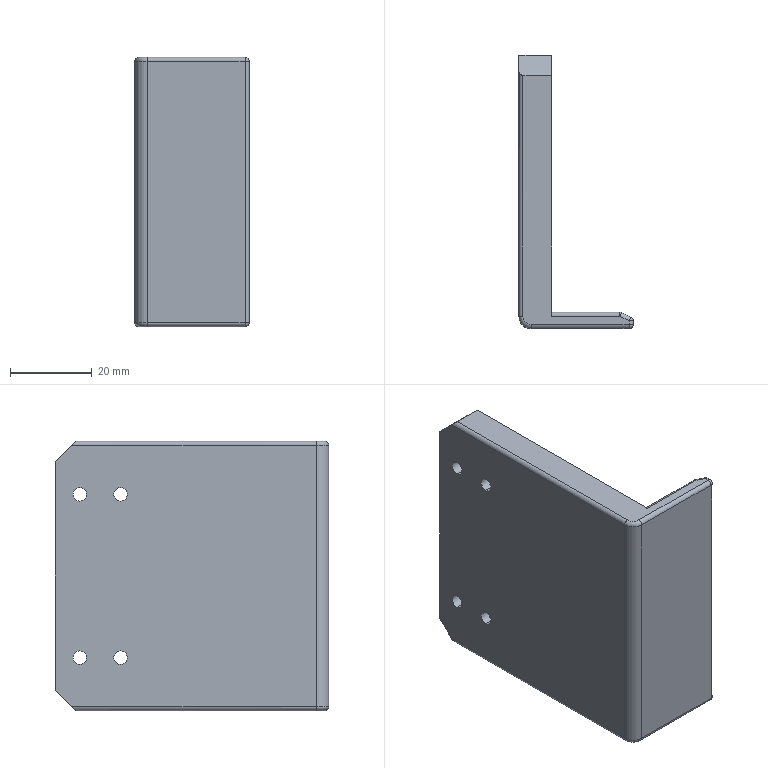Part | SolidWorks | features Fillet 3, Chamfer 2, Extrusion 1, HoleWzd 1 | 1 solid | 41 faces | box 28 x 67 x 66 mm | volume 39840 mm3 | cylinder 22 | plane 11 | sphere 6 | torus 2 | commonest cylinder face diameters 2 x13 3.3 x8 6 x1
STEP:
#1=CARTESIAN_POINT('',(8.,61.,-21.65));
#2=VERTEX_POINT('',#1);
#3=CARTESIAN_POINT('',(8.,61.,-18.35));
#4=VERTEX_POINT('',#3);
#5=CARTESIAN_POINT('',(8.,61.,-20.));
#6=DIRECTION('',(-1.,0.,0.));
#7=DIRECTION('',(0.,0.,1.));
#8=AXIS2_PLACEMENT_3D('',#5,#6,#7);
#9=CIRCLE('',#8,1.65);
#10=EDGE_CURVE('',#2,#4,#9,.T.);
#11=ORIENTED_EDGE('',*,*,#10,.F.);
#12=CARTESIAN_POINT('',(0.,61.,-21.65));
#13=VERTEX_POINT('',#12);
#14=CARTESIAN_POINT('',(0.,61.,-21.65));
#15=DIRECTION('',(-1.,0.,0.));
#16=VECTOR('',#15,1000.);
#17=LINE('',#14,#16);
#18=EDGE_CURVE('',#2,#13,#17,.T.);
#19=ORIENTED_EDGE('',*,*,#18,.T.);
#20=CARTESIAN_POINT('',(0.,61.,-18.35));
#21=VERTEX_POINT('',#20);
#22=CARTESIAN_POINT('',(0.,61.,-20.));
#23=DIRECTION('',(-1.,0.,0.));
#24=DIRECTION('',(0.,0.,1.));
#25=AXIS2_PLACEMENT_3D('',#22,#23,#24);
#26=CIRCLE('',#25,1.65);
#27=EDGE_CURVE('',#13,#21,#26,.T.);
#28=ORIENTED_EDGE('',*,*,#27,.T.);
#29=CARTESIAN_POINT('',(0.,61.,-18.35));
#30=DIRECTION('',(-1.,0.,0.));
#31=VECTOR('',#30,1000.);
#32=LINE('',#29,#31);
#33=EDGE_CURVE('',#4,#21,#32,.T.);
#34=ORIENTED_EDGE('',*,*,#33,.F.);
#35=EDGE_LOOP('',(#11,#19,#28,#34));
#36=FACE_OUTER_BOUND('',#35,.T.);
#37=CARTESIAN_POINT('',(0.,61.,-20.));
#38=DIRECTION('',(-1.,0.,0.));
#39=DIRECTION('',(0.,0.,1.));
#40=AXIS2_PLACEMENT_3D('',#37,#38,#39);
#41=CYLINDRICAL_SURFACE('',#40,1.65);
#42=ADVANCED_FACE('',(#36),#41,.F.);
#43=CARTESIAN_POINT('',(8.,61.,18.35));
#44=VERTEX_POINT('',#43);
#45=CARTESIAN_POINT('',(8.,61.,21.65));
#46=VERTEX_POINT('',#45);
#47=CARTESIAN_POINT('',(8.,61.,20.));
#48=DIRECTION('',(-1.,0.,0.));
#49=DIRECTION('',(0.,0.,1.));
#50=AXIS2_PLACEMENT_3D('',#47,#48,#49);
#51=CIRCLE('',#50,1.65);
#52=EDGE_CURVE('',#44,#46,#51,.T.);
#53=ORIENTED_EDGE('',*,*,#52,.F.);
#54=CARTESIAN_POINT('',(0.,61.,18.35));
#55=VERTEX_POINT('',#54);
#56=CARTESIAN_POINT('',(0.,61.,18.35));
#57=DIRECTION('',(-1.,0.,0.));
#58=VECTOR('',#57,1000.);
#59=LINE('',#56,#58);
#60=EDGE_CURVE('',#44,#55,#59,.T.);
#61=ORIENTED_EDGE('',*,*,#60,.T.);
#62=CARTESIAN_POINT('',(0.,61.,21.65));
#63=VERTEX_POINT('',#62);
#64=CARTESIAN_POINT('',(0.,61.,20.));
#65=DIRECTION('',(-1.,0.,0.));
#66=DIRECTION('',(0.,0.,1.));
#67=AXIS2_PLACEMENT_3D('',#64,#65,#66);
#68=CIRCLE('',#67,1.65);
#69=EDGE_CURVE('',#55,#63,#68,.T.);
#70=ORIENTED_EDGE('',*,*,#69,.T.);
#71=CARTESIAN_POINT('',(0.,61.,21.65));
#72=DIRECTION('',(-1.,0.,0.));
#73=VECTOR('',#72,1000.);
#74=LINE('',#71,#73);
#75=EDGE_CURVE('',#46,#63,#74,.T.);
#76=ORIENTED_EDGE('',*,*,#75,.F.);
#77=EDGE_LOOP('',(#53,#61,#70,#76));
#78=FACE_OUTER_BOUND('',#77,.T.);
#79=CARTESIAN_POINT('',(0.,61.,20.));
#80=DIRECTION('',(-1.,0.,0.));
#81=DIRECTION('',(0.,0.,1.));
#82=AXIS2_PLACEMENT_3D('',#79,#80,#81);
#83=CYLINDRICAL_SURFACE('',#82,1.65);
#84=ADVANCED_FACE('',(#78),#83,.F.);
#85=CARTESIAN_POINT('',(8.,51.,-21.65));
#86=VERTEX_POINT('',#85);
#87=CARTESIAN_POINT('',(8.,51.,-18.35));
#88=VERTEX_POINT('',#87);
#89=CARTESIAN_POINT('',(8.,51.,-20.));
#90=DIRECTION('',(-1.,0.,0.));
#91=DIRECTION('',(0.,0.,1.));
#92=AXIS2_PLACEMENT_3D('',#89,#90,#91);
#93=CIRCLE('',#92,1.65);
#94=EDGE_CURVE('',#86,#88,#93,.T.);
#95=ORIENTED_EDGE('',*,*,#94,.F.);
#96=CARTESIAN_POINT('',(0.,51.,-21.65));
#97=VERTEX_POINT('',#96);
#98=CARTESIAN_POINT('',(0.,51.,-21.65));
#99=DIRECTION('',(-1.,0.,0.));
#100=VECTOR('',#99,1000.);
#101=LINE('',#98,#100);
#102=EDGE_CURVE('',#86,#97,#101,.T.);
#103=ORIENTED_EDGE('',*,*,#102,.T.);
#104=CARTESIAN_POINT('',(0.,51.,-18.35));
#105=VERTEX_POINT('',#104);
#106=CARTESIAN_POINT('',(0.,51.,-20.));
#107=DIRECTION('',(-1.,0.,0.));
#108=DIRECTION('',(0.,0.,1.));
#109=AXIS2_PLACEMENT_3D('',#106,#107,#108);
#110=CIRCLE('',#109,1.65);
#111=EDGE_CURVE('',#97,#105,#110,.T.);
#112=ORIENTED_EDGE('',*,*,#111,.T.);
#113=CARTESIAN_POINT('',(0.,51.,-18.35));
#114=DIRECTION('',(-1.,0.,0.));
#115=VECTOR('',#114,1000.);
#116=LINE('',#113,#115);
#117=EDGE_CURVE('',#88,#105,#116,.T.);
#118=ORIENTED_EDGE('',*,*,#117,.F.);
#119=EDGE_LOOP('',(#95,#103,#112,#118));
#120=FACE_OUTER_BOUND('',#119,.T.);
#121=CARTESIAN_POINT('',(0.,51.,-20.));
#122=DIRECTION('',(-1.,0.,0.));
#123=DIRECTION('',(0.,0.,1.));
#124=AXIS2_PLACEMENT_3D('',#121,#122,#123);
#125=CYLINDRICAL_SURFACE('',#124,1.65);
#126=ADVANCED_FACE('',(#120),#125,.F.);
#127=CARTESIAN_POINT('',(8.,51.,18.35));
#128=VERTEX_POINT('',#127);
#129=CARTESIAN_POINT('',(8.,51.,21.65));
#130=VERTEX_POINT('',#129);
#131=CARTESIAN_POINT('',(8.,51.,20.));
#132=DIRECTION('',(-1.,0.,0.));
#133=DIRECTION('',(0.,0.,1.));
#134=AXIS2_PLACEMENT_3D('',#131,#132,#133);
#135=CIRCLE('',#134,1.65);
#136=EDGE_CURVE('',#128,#130,#135,.T.);
#137=ORIENTED_EDGE('',*,*,#136,.F.);
#138=CARTESIAN_POINT('',(0.,51.,18.35));
#139=VERTEX_POINT('',#138);
#140=CARTESIAN_POINT('',(0.,51.,18.35));
#141=DIRECTION('',(-1.,0.,0.));
#142=VECTOR('',#141,1000.);
#143=LINE('',#140,#142);
#144=EDGE_CURVE('',#128,#139,#143,.T.);
#145=ORIENTED_EDGE('',*,*,#144,.T.);
#146=CARTESIAN_POINT('',(0.,51.,21.65));
#147=VERTEX_POINT('',#146);
#148=CARTESIAN_POINT('',(0.,51.,20.));
#149=DIRECTION('',(-1.,0.,0.));
#150=DIRECTION('',(0.,0.,1.));
#151=AXIS2_PLACEMENT_3D('',#148,#149,#150);
#152=CIRCLE('',#151,1.65);
#153=EDGE_CURVE('',#139,#147,#152,.T.);
#154=ORIENTED_EDGE('',*,*,#153,.T.);
#155=CARTESIAN_POINT('',(0.,51.,21.65));
#156=DIRECTION('',(-1.,0.,0.));
#157=VECTOR('',#156,1000.);
#158=LINE('',#155,#157);
#159=EDGE_CURVE('',#130,#147,#158,.T.);
#160=ORIENTED_EDGE('',*,*,#159,.F.);
#161=EDGE_LOOP('',(#137,#145,#154,#160));
#162=FACE_OUTER_BOUND('',#161,.T.);
#163=CARTESIAN_POINT('',(0.,51.,20.));
#164=DIRECTION('',(-1.,0.,0.));
#165=DIRECTION('',(0.,0.,1.));
#166=AXIS2_PLACEMENT_3D('',#163,#164,#165);
#167=CYLINDRICAL_SURFACE('',#166,1.65);
#168=ADVANCED_FACE('',(#162),#167,.F.);
#169=CARTESIAN_POINT('',(27.,0.,-32.));
#170=VERTEX_POINT('',#169);
#171=CARTESIAN_POINT('',(27.,0.,32.));
#172=VERTEX_POINT('',#171);
#173=CARTESIAN_POINT('',(27.,0.,33.));
#174=DIRECTION('',(0.,0.,1.));
#175=VECTOR('',#174,1000.);
#176=LINE('',#173,#175);
#177=EDGE_CURVE('',#170,#172,#176,.T.);
#178=ORIENTED_EDGE('',*,*,#177,.T.);
#179=CARTESIAN_POINT('',(3.,0.,32.));
#180=VERTEX_POINT('',#179);
#181=CARTESIAN_POINT('',(3.,0.,32.));
#182=DIRECTION('',(-1.,0.,0.));
#183=VECTOR('',#182,1000.);
#184=LINE('',#181,#183);
#185=EDGE_CURVE('',#172,#180,#184,.T.);
#186=ORIENTED_EDGE('',*,*,#185,.T.);
#187=CARTESIAN_POINT('',(3.,0.,-32.));
#188=VERTEX_POINT('',#187);
#189=CARTESIAN_POINT('',(3.,0.,33.));
#190=DIRECTION('',(0.,0.,-1.));
#191=VECTOR('',#190,1000.);
#192=LINE('',#189,#191);
#193=EDGE_CURVE('',#180,#188,#192,.T.);
#194=ORIENTED_EDGE('',*,*,#193,.T.);
#195=CARTESIAN_POINT('',(0.,0.,-32.));
#196=DIRECTION('',(1.,0.,0.));
#197=VECTOR('',#196,1000.);
#198=LINE('',#195,#197);
#199=EDGE_CURVE('',#188,#170,#198,.T.);
#200=ORIENTED_EDGE('',*,*,#199,.T.);
#201=EDGE_LOOP('',(#178,#186,#194,#200));
#202=FACE_OUTER_BOUND('',#201,.T.);
#203=CARTESIAN_POINT('',(0.,0.,33.));
#204=DIRECTION('',(0.,1.,0.));
#205=DIRECTION('',(0.,0.,1.));
#206=AXIS2_PLACEMENT_3D('',#203,#204,#205);
#207=PLANE('',#206);
#208=ADVANCED_FACE('',(#202),#207,.F.);
#209=CARTESIAN_POINT('',(28.,1.882,-32.));
#210=VERTEX_POINT('',#209);
#211=CARTESIAN_POINT('',(28.,1.882,32.));
#212=VERTEX_POINT('',#211);
#213=CARTESIAN_POINT('',(28.,1.882,33.));
#214=DIRECTION('',(0.,0.,1.));
#215=VECTOR('',#214,1000.);
#216=LINE('',#213,#215);
#217=EDGE_CURVE('',#210,#212,#216,.T.);
#218=ORIENTED_EDGE('',*,*,#217,.T.);
#219=CARTESIAN_POINT('',(28.,1.,32.));
#220=VERTEX_POINT('',#219);
#221=CARTESIAN_POINT('',(28.,1.,32.));
#222=DIRECTION('',(0.,-1.,0.));
#223=VECTOR('',#222,1000.);
#224=LINE('',#221,#223);
#225=EDGE_CURVE('',#212,#220,#224,.T.);
#226=ORIENTED_EDGE('',*,*,#225,.T.);
#227=CARTESIAN_POINT('',(28.,1.,-32.));
#228=VERTEX_POINT('',#227);
#229=CARTESIAN_POINT('',(28.,1.,33.));
#230=DIRECTION('',(0.,0.,-1.));
#231=VECTOR('',#230,1000.);
#232=LINE('',#229,#231);
#233=EDGE_CURVE('',#220,#228,#232,.T.);
#234=ORIENTED_EDGE('',*,*,#233,.T.);
#235=CARTESIAN_POINT('',(28.,0.,-32.));
#236=DIRECTION('',(0.,1.,0.));
#237=VECTOR('',#236,1000.);
#238=LINE('',#235,#237);
#239=EDGE_CURVE('',#228,#210,#238,.T.);
#240=ORIENTED_EDGE('',*,*,#239,.T.);
#241=EDGE_LOOP('',(#218,#226,#234,#240));
#242=FACE_OUTER_BOUND('',#241,.T.);
#243=CARTESIAN_POINT('',(28.,0.,33.));
#244=DIRECTION('',(-1.,0.,0.));
#245=DIRECTION('',(0.,0.,1.));
#246=AXIS2_PLACEMENT_3D('',#243,#244,#245);
#247=PLANE('',#246);
#248=ADVANCED_FACE('',(#242),#247,.F.);
#249=CARTESIAN_POINT('',(8.,4.,32.));
#250=VERTEX_POINT('',#249);
#251=CARTESIAN_POINT('',(8.,4.,-32.));
#252=VERTEX_POINT('',#251);
#253=CARTESIAN_POINT('',(8.,4.,33.));
#254=DIRECTION('',(0.,0.,-1.));
#255=VECTOR('',#254,1000.);
#256=LINE('',#253,#255);
#257=EDGE_CURVE('',#250,#252,#256,.T.);
#258=ORIENTED_EDGE('',*,*,#257,.F.);
#259=CARTESIAN_POINT('',(24.764,4.,32.));
#260=VERTEX_POINT('',#259);
#261=CARTESIAN_POINT('',(24.764,4.,32.));
#262=DIRECTION('',(1.,0.,0.));
#263=VECTOR('',#262,1000.);
#264=LINE('',#261,#263);
#265=EDGE_CURVE('',#250,#260,#264,.T.);
#266=ORIENTED_EDGE('',*,*,#265,.T.);
#267=CARTESIAN_POINT('',(24.764,4.,-32.));
#268=VERTEX_POINT('',#267);
#269=CARTESIAN_POINT('',(24.764,4.,-33.));
#270=DIRECTION('',(0.,0.,-1.));
#271=VECTOR('',#270,1000.);
#272=LINE('',#269,#271);
#273=EDGE_CURVE('',#260,#268,#272,.T.);
#274=ORIENTED_EDGE('',*,*,#273,.T.);
#275=CARTESIAN_POINT('',(28.,4.,-32.));
#276=DIRECTION('',(-1.,0.,0.));
#277=VECTOR('',#276,1000.);
#278=LINE('',#275,#277);
#279=EDGE_CURVE('',#268,#252,#278,.T.);
#280=ORIENTED_EDGE('',*,*,#279,.T.);
#281=EDGE_LOOP('',(#258,#266,#274,#280));
#282=FACE_OUTER_BOUND('',#281,.T.);
#283=CARTESIAN_POINT('',(28.,4.,33.));
#284=DIRECTION('',(0.,-1.,0.));
#285=DIRECTION('',(1.,0.,0.));
#286=AXIS2_PLACEMENT_3D('',#283,#284,#285);
#287=PLANE('',#286);
#288=ADVANCED_FACE('',(#282),#287,.F.);
#289=CARTESIAN_POINT('',(8.,61.,-20.));
#290=DIRECTION('',(-1.,0.,0.));
#291=DIRECTION('',(0.,0.,1.));
#292=AXIS2_PLACEMENT_3D('',#289,#290,#291);
#293=CIRCLE('',#292,1.65);
#294=EDGE_CURVE('',#4,#2,#293,.T.);
#295=ORIENTED_EDGE('',*,*,#294,.T.);
#296=ORIENTED_EDGE('',*,*,#10,.T.);
#297=EDGE_LOOP('',(#295,#296));
#298=FACE_BOUND('',#297,.T.);
#299=CARTESIAN_POINT('',(8.,61.,20.));
#300=DIRECTION('',(-1.,0.,0.));
#301=DIRECTION('',(0.,0.,1.));
#302=AXIS2_PLACEMENT_3D('',#299,#300,#301);
#303=CIRCLE('',#302,1.65);
#304=EDGE_CURVE('',#46,#44,#303,.T.);
#305=ORIENTED_EDGE('',*,*,#304,.T.);
#306=ORIENTED_EDGE('',*,*,#52,.T.);
#307=EDGE_LOOP('',(#305,#306));
#308=FACE_BOUND('',#307,.T.);
#309=CARTESIAN_POINT('',(8.,51.,-20.));
#310=DIRECTION('',(-1.,0.,0.));
#311=DIRECTION('',(0.,0.,1.));
#312=AXIS2_PLACEMENT_3D('',#309,#310,#311);
#313=CIRCLE('',#312,1.65);
#314=EDGE_CURVE('',#88,#86,#313,.T.);
#315=ORIENTED_EDGE('',*,*,#314,.T.);
#316=ORIENTED_EDGE('',*,*,#94,.T.);
#317=EDGE_LOOP('',(#315,#316));
#318=FACE_BOUND('',#317,.T.);
#319=CARTESIAN_POINT('',(8.,51.,20.));
#320=DIRECTION('',(-1.,0.,0.));
#321=DIRECTION('',(0.,0.,1.));
#322=AXIS2_PLACEMENT_3D('',#319,#320,#321);
#323=CIRCLE('',#322,1.65);
#324=EDGE_CURVE('',#130,#128,#323,.T.);
#325=ORIENTED_EDGE('',*,*,#324,.T.);
#326=ORIENTED_EDGE('',*,*,#136,.T.);
#327=EDGE_LOOP('',(#325,#326));
#328=FACE_BOUND('',#327,.T.);
#329=CARTESIAN_POINT('',(8.,67.,28.));
#330=VERTEX_POINT('',#329);
#331=CARTESIAN_POINT('',(8.,67.,-28.));
#332=VERTEX_POINT('',#331);
#333=CARTESIAN_POINT('',(8.,67.,33.));
#334=DIRECTION('',(0.,0.,-1.));
#335=VECTOR('',#334,1000.);
#336=LINE('',#333,#335);
#337=EDGE_CURVE('',#330,#332,#336,.T.);
#338=ORIENTED_EDGE('',*,*,#337,.F.);
#339=CARTESIAN_POINT('',(8.,62.,33.));
#340=VERTEX_POINT('',#339);
#341=CARTESIAN_POINT('',(8.,62.,33.));
#342=DIRECTION('',(0.,-0.7071,0.7071));
#343=VECTOR('',#342,1000.);
#344=LINE('',#341,#343);
#345=EDGE_CURVE('',#330,#340,#344,.T.);
#346=ORIENTED_EDGE('',*,*,#345,.T.);
#347=CARTESIAN_POINT('',(8.,3.,33.));
#348=VERTEX_POINT('',#347);
#349=CARTESIAN_POINT('',(8.,4.,33.));
#350=DIRECTION('',(0.,1.,0.));
#351=VECTOR('',#350,1000.);
#352=LINE('',#349,#351);
#353=EDGE_CURVE('',#348,#340,#352,.T.);
#354=ORIENTED_EDGE('',*,*,#353,.F.);
#355=CARTESIAN_POINT('',(8.,3.,32.));
#356=DIRECTION('',(-1.,0.,0.));
#357=DIRECTION('',(0.,0.,1.));
#358=AXIS2_PLACEMENT_3D('',#355,#356,#357);
#359=CIRCLE('',#358,1.);
#360=EDGE_CURVE('',#348,#250,#359,.T.);
#361=ORIENTED_EDGE('',*,*,#360,.T.);
#362=ORIENTED_EDGE('',*,*,#257,.T.);
#363=CARTESIAN_POINT('',(8.,3.,-33.));
#364=VERTEX_POINT('',#363);
#365=CARTESIAN_POINT('',(8.,3.,-32.));
#366=DIRECTION('',(-1.,0.,0.));
#367=DIRECTION('',(0.,0.,1.));
#368=AXIS2_PLACEMENT_3D('',#365,#366,#367);
#369=CIRCLE('',#368,1.);
#370=EDGE_CURVE('',#252,#364,#369,.T.);
#371=ORIENTED_EDGE('',*,*,#370,.T.);
#372=CARTESIAN_POINT('',(8.,62.,-33.));
#373=VERTEX_POINT('',#372);
#374=CARTESIAN_POINT('',(8.,4.,-33.));
#375=DIRECTION('',(0.,1.,0.));
#376=VECTOR('',#375,1000.);
#377=LINE('',#374,#376);
#378=EDGE_CURVE('',#364,#373,#377,.T.);
#379=ORIENTED_EDGE('',*,*,#378,.T.);
#380=CARTESIAN_POINT('',(8.,67.,-28.));
#381=DIRECTION('',(0.,0.7071,0.7071));
#382=VECTOR('',#381,1000.);
#383=LINE('',#380,#382);
#384=EDGE_CURVE('',#373,#332,#383,.T.);
#385=ORIENTED_EDGE('',*,*,#384,.T.);
#386=EDGE_LOOP('',(#338,#346,#354,#361,#362,#371,#379,#385));
#387=FACE_OUTER_BOUND('',#386,.T.);
#388=CARTESIAN_POINT('',(8.,4.,33.));
#389=DIRECTION('',(-1.,0.,0.));
#390=DIRECTION('',(0.,0.,1.));
#391=AXIS2_PLACEMENT_3D('',#388,#389,#390);
#392=PLANE('',#391);
#393=ADVANCED_FACE('',(#298,#308,#318,#328,#387),#392,.F.);
#394=CARTESIAN_POINT('',(0.,67.,28.));
#395=VERTEX_POINT('',#394);
#396=CARTESIAN_POINT('',(0.,67.,-28.));
#397=VERTEX_POINT('',#396);
#398=CARTESIAN_POINT('',(0.,67.,33.));
#399=DIRECTION('',(0.,0.,-1.));
#400=VECTOR('',#399,1000.);
#401=LINE('',#398,#400);
#402=EDGE_CURVE('',#395,#397,#401,.T.);
#403=ORIENTED_EDGE('',*,*,#402,.F.);
#404=CARTESIAN_POINT('',(8.,67.,28.));
#405=DIRECTION('',(1.,0.,0.));
#406=VECTOR('',#405,1000.);
#407=LINE('',#404,#406);
#408=EDGE_CURVE('',#395,#330,#407,.T.);
#409=ORIENTED_EDGE('',*,*,#408,.T.);
#410=ORIENTED_EDGE('',*,*,#337,.T.);
#411=CARTESIAN_POINT('',(8.,67.,-28.));
#412=DIRECTION('',(-1.,0.,0.));
#413=VECTOR('',#412,1000.);
#414=LINE('',#411,#413);
#415=EDGE_CURVE('',#332,#397,#414,.T.);
#416=ORIENTED_EDGE('',*,*,#415,.T.);
#417=EDGE_LOOP('',(#403,#409,#410,#416));
#418=FACE_OUTER_BOUND('',#417,.T.);
#419=CARTESIAN_POINT('',(8.,67.,33.));
#420=DIRECTION('',(0.,-1.,0.));
#421=DIRECTION('',(0.,0.,-1.));
#422=AXIS2_PLACEMENT_3D('',#419,#420,#421);
#423=PLANE('',#422);
#424=ADVANCED_FACE('',(#418),#423,.F.);
#425=CARTESIAN_POINT('',(0.,61.,-20.));
#426=DIRECTION('',(-1.,0.,0.));
#427=DIRECTION('',(0.,0.,1.));
#428=AXIS2_PLACEMENT_3D('',#425,#426,#427);
#429=CIRCLE('',#428,1.65);
#430=EDGE_CURVE('',#21,#13,#429,.T.);
#431=ORIENTED_EDGE('',*,*,#430,.F.);
#432=ORIENTED_EDGE('',*,*,#27,.F.);
#433=EDGE_LOOP('',(#431,#432));
#434=FACE_BOUND('',#433,.T.);
#435=CARTESIAN_POINT('',(0.,61.,20.));
#436=DIRECTION('',(-1.,0.,0.));
#437=DIRECTION('',(0.,0.,1.));
#438=AXIS2_PLACEMENT_3D('',#435,#436,#437);
#439=CIRCLE('',#438,1.65);
#440=EDGE_CURVE('',#63,#55,#439,.T.);
#441=ORIENTED_EDGE('',*,*,#440,.F.);
#442=ORIENTED_EDGE('',*,*,#69,.F.);
#443=EDGE_LOOP('',(#441,#442));
#444=FACE_BOUND('',#443,.T.);
#445=CARTESIAN_POINT('',(0.,51.,-20.));
#446=DIRECTION('',(-1.,0.,0.));
#447=DIRECTION('',(0.,0.,1.));
#448=AXIS2_PLACEMENT_3D('',#445,#446,#447);
#449=CIRCLE('',#448,1.65);
#450=EDGE_CURVE('',#105,#97,#449,.T.);
#451=ORIENTED_EDGE('',*,*,#450,.F.);
#452=ORIENTED_EDGE('',*,*,#111,.F.);
#453=EDGE_LOOP('',(#451,#452));
#454=FACE_BOUND('',#453,.T.);
#455=CARTESIAN_POINT('',(0.,51.,20.));
#456=DIRECTION('',(-1.,0.,0.));
#457=DIRECTION('',(0.,0.,1.));
#458=AXIS2_PLACEMENT_3D('',#455,#456,#457);
#459=CIRCLE('',#458,1.65);
#460=EDGE_CURVE('',#147,#139,#459,.T.);
#461=ORIENTED_EDGE('',*,*,#460,.F.);
#462=ORIENTED_EDGE('',*,*,#153,.F.);
#463=EDGE_LOOP('',(#461,#462));
#464=FACE_BOUND('',#463,.T.);
#465=CARTESIAN_POINT('',(0.,3.,-32.));
#466=VERTEX_POINT('',#465);
#467=CARTESIAN_POINT('',(0.,3.,32.));
#468=VERTEX_POINT('',#467);
#469=CARTESIAN_POINT('',(0.,3.,33.));
#470=DIRECTION('',(0.,0.,1.));
#471=VECTOR('',#470,1000.);
#472=LINE('',#469,#471);
#473=EDGE_CURVE('',#466,#468,#472,.T.);
#474=ORIENTED_EDGE('',*,*,#473,.T.);
#475=CARTESIAN_POINT('',(0.,63.,32.));
#476=VERTEX_POINT('',#475);
#477=CARTESIAN_POINT('',(0.,62.,32.));
#478=DIRECTION('',(0.,1.,0.));
#479=VECTOR('',#478,1000.);
#480=LINE('',#477,#479);
#481=EDGE_CURVE('',#468,#476,#480,.T.);
#482=ORIENTED_EDGE('',*,*,#481,.T.);
#483=CARTESIAN_POINT('',(0.,62.,33.));
#484=DIRECTION('',(0.,0.7071,-0.7071));
#485=VECTOR('',#484,1000.);
#486=LINE('',#483,#485);
#487=EDGE_CURVE('',#476,#395,#486,.T.);
#488=ORIENTED_EDGE('',*,*,#487,.T.);
#489=ORIENTED_EDGE('',*,*,#402,.T.);
#490=CARTESIAN_POINT('',(0.,63.,-32.));
#491=VERTEX_POINT('',#490);
#492=CARTESIAN_POINT('',(0.,67.,-28.));
#493=DIRECTION('',(0.,-0.7071,-0.7071));
#494=VECTOR('',#493,1000.);
#495=LINE('',#492,#494);
#496=EDGE_CURVE('',#397,#491,#495,.T.);
#497=ORIENTED_EDGE('',*,*,#496,.T.);
#498=CARTESIAN_POINT('',(0.,67.,-32.));
#499=DIRECTION('',(0.,-1.,0.));
#500=VECTOR('',#499,1000.);
#501=LINE('',#498,#500);
#502=EDGE_CURVE('',#491,#466,#501,.T.);
#503=ORIENTED_EDGE('',*,*,#502,.T.);
#504=EDGE_LOOP('',(#474,#482,#488,#489,#497,#503));
#505=FACE_OUTER_BOUND('',#504,.T.);
#506=CARTESIAN_POINT('',(0.,67.,33.));
#507=DIRECTION('',(1.,0.,0.));
#508=DIRECTION('',(0.,0.,-1.));
#509=AXIS2_PLACEMENT_3D('',#506,#507,#508);
#510=PLANE('',#509);
#511=ADVANCED_FACE('',(#434,#444,#454,#464,#505),#510,.F.);
#512=CARTESIAN_POINT('',(1.,62.,33.));
#513=VERTEX_POINT('',#512);
#514=CARTESIAN_POINT('',(0.,62.,33.));
#515=DIRECTION('',(-1.,0.,0.));
#516=VECTOR('',#515,1000.);
#517=LINE('',#514,#516);
#518=EDGE_CURVE('',#340,#513,#517,.T.);
#519=ORIENTED_EDGE('',*,*,#518,.T.);
#520=CARTESIAN_POINT('',(1.,3.,33.));
#521=VERTEX_POINT('',#520);
#522=CARTESIAN_POINT('',(1.,3.,33.));
#523=DIRECTION('',(0.,-1.,0.));
#524=VECTOR('',#523,1000.);
#525=LINE('',#522,#524);
#526=EDGE_CURVE('',#513,#521,#525,.T.);
#527=ORIENTED_EDGE('',*,*,#526,.T.);
#528=CARTESIAN_POINT('',(3.,1.,33.));
#529=VERTEX_POINT('',#528);
#530=CARTESIAN_POINT('',(3.,3.,33.));
#531=DIRECTION('',(0.,0.,1.));
#532=DIRECTION('',(1.,0.,0.));
#533=AXIS2_PLACEMENT_3D('',#530,#531,#532);
#534=CIRCLE('',#533,2.);
#535=EDGE_CURVE('',#521,#529,#534,.T.);
#536=ORIENTED_EDGE('',*,*,#535,.T.);
#537=CARTESIAN_POINT('',(27.,1.,33.));
#538=VERTEX_POINT('',#537);
#539=CARTESIAN_POINT('',(27.,1.,33.));
#540=DIRECTION('',(1.,0.,0.));
#541=VECTOR('',#540,1000.);
#542=LINE('',#539,#541);
#543=EDGE_CURVE('',#529,#538,#542,.T.);
#544=ORIENTED_EDGE('',*,*,#543,.T.);
#545=CARTESIAN_POINT('',(27.,1.882,33.));
#546=VERTEX_POINT('',#545);
#547=CARTESIAN_POINT('',(27.,1.882,33.));
#548=DIRECTION('',(0.,1.,0.));
#549=VECTOR('',#548,1000.);
#550=LINE('',#547,#549);
#551=EDGE_CURVE('',#538,#546,#550,.T.);
#552=ORIENTED_EDGE('',*,*,#551,.T.);
#553=CARTESIAN_POINT('',(24.764,3.,33.));
#554=VERTEX_POINT('',#553);
#555=CARTESIAN_POINT('',(6.153,12.306,33.));
#556=DIRECTION('',(-0.8944,0.4472,0.));
#557=VECTOR('',#556,1000.);
#558=LINE('',#555,#557);
#559=EDGE_CURVE('',#546,#554,#558,.T.);
#560=ORIENTED_EDGE('',*,*,#559,.T.);
#561=CARTESIAN_POINT('',(8.,3.,33.));
#562=DIRECTION('',(-1.,0.,0.));
#563=VECTOR('',#562,1000.);
#564=LINE('',#561,#563);
#565=EDGE_CURVE('',#554,#348,#564,.T.);
#566=ORIENTED_EDGE('',*,*,#565,.T.);
#567=ORIENTED_EDGE('',*,*,#353,.T.);
#568=EDGE_LOOP('',(#519,#527,#536,#544,#552,#560,#566,#567));
#569=FACE_OUTER_BOUND('',#568,.T.);
#570=CARTESIAN_POINT('',(0.,0.,33.));
#571=DIRECTION('',(0.,0.,1.));
#572=DIRECTION('',(1.,0.,0.));
#573=AXIS2_PLACEMENT_3D('',#570,#571,#572);
#574=PLANE('',#573);
#575=ADVANCED_FACE('',(#569),#574,.T.);
#576=CARTESIAN_POINT('',(3.,1.,-33.));
#577=VERTEX_POINT('',#576);
#578=CARTESIAN_POINT('',(1.,3.,-33.));
#579=VERTEX_POINT('',#578);
#580=CARTESIAN_POINT('',(3.,3.,-33.));
#581=DIRECTION('',(0.,0.,-1.));
#582=DIRECTION('',(1.,0.,0.));
#583=AXIS2_PLACEMENT_3D('',#580,#581,#582);
#584=CIRCLE('',#583,2.);
#585=EDGE_CURVE('',#577,#579,#584,.T.);
#586=ORIENTED_EDGE('',*,*,#585,.T.);
#587=CARTESIAN_POINT('',(1.,62.,-33.));
#588=VERTEX_POINT('',#587);
#589=CARTESIAN_POINT('',(1.,0.,-33.));
#590=DIRECTION('',(0.,1.,0.));
#591=VECTOR('',#590,1000.);
#592=LINE('',#589,#591);
#593=EDGE_CURVE('',#579,#588,#592,.T.);
#594=ORIENTED_EDGE('',*,*,#593,.T.);
#595=CARTESIAN_POINT('',(0.,62.,-33.));
#596=DIRECTION('',(1.,0.,0.));
#597=VECTOR('',#596,1000.);
#598=LINE('',#595,#597);
#599=EDGE_CURVE('',#588,#373,#598,.T.);
#600=ORIENTED_EDGE('',*,*,#599,.T.);
#601=ORIENTED_EDGE('',*,*,#378,.F.);
#602=CARTESIAN_POINT('',(24.764,3.,-33.));
#603=VERTEX_POINT('',#602);
#604=CARTESIAN_POINT('',(0.,3.,-33.));
#605=DIRECTION('',(1.,0.,0.));
#606=VECTOR('',#605,1000.);
#607=LINE('',#604,#606);
#608=EDGE_CURVE('',#364,#603,#607,.T.);
#609=ORIENTED_EDGE('',*,*,#608,.T.);
#610=CARTESIAN_POINT('',(27.,1.882,-33.));
#611=VERTEX_POINT('',#610);
#612=CARTESIAN_POINT('',(27.,1.882,-33.));
#613=DIRECTION('',(0.8944,-0.4472,0.));
#614=VECTOR('',#613,1000.);
#615=LINE('',#612,#614);
#616=EDGE_CURVE('',#603,#611,#615,.T.);
#617=ORIENTED_EDGE('',*,*,#616,.T.);
#618=CARTESIAN_POINT('',(27.,1.,-33.));
#619=VERTEX_POINT('',#618);
#620=CARTESIAN_POINT('',(27.,0.,-33.));
#621=DIRECTION('',(0.,-1.,0.));
#622=VECTOR('',#621,1000.);
#623=LINE('',#620,#622);
#624=EDGE_CURVE('',#611,#619,#623,.T.);
#625=ORIENTED_EDGE('',*,*,#624,.T.);
#626=CARTESIAN_POINT('',(0.,1.,-33.));
#627=DIRECTION('',(-1.,0.,0.));
#628=VECTOR('',#627,1000.);
#629=LINE('',#626,#628);
#630=EDGE_CURVE('',#619,#577,#629,.T.);
#631=ORIENTED_EDGE('',*,*,#630,.T.);
#632=EDGE_LOOP('',(#586,#594,#600,#601,#609,#617,#625,#631));
#633=FACE_OUTER_BOUND('',#632,.T.);
#634=CARTESIAN_POINT('',(0.,0.,-33.));
#635=DIRECTION('',(0.,0.,1.));
#636=DIRECTION('',(1.,0.,0.));
#637=AXIS2_PLACEMENT_3D('',#634,#635,#636);
#638=PLANE('',#637);
#639=ADVANCED_FACE('',(#633),#638,.F.);
#640=CARTESIAN_POINT('',(25.211,3.894,-32.));
#641=VERTEX_POINT('',#640);
#642=CARTESIAN_POINT('',(25.211,3.894,32.));
#643=VERTEX_POINT('',#642);
#644=CARTESIAN_POINT('',(25.211,3.894,33.));
#645=DIRECTION('',(0.,0.,1.));
#646=VECTOR('',#645,1000.);
#647=LINE('',#644,#646);
#648=EDGE_CURVE('',#641,#643,#647,.T.);
#649=ORIENTED_EDGE('',*,*,#648,.T.);
#650=CARTESIAN_POINT('',(27.447,2.776,32.));
#651=VERTEX_POINT('',#650);
#652=CARTESIAN_POINT('',(25.,4.,32.));
#653=DIRECTION('',(0.8944,-0.4472,0.));
#654=VECTOR('',#653,1000.);
#655=LINE('',#652,#654);
#656=EDGE_CURVE('',#643,#651,#655,.T.);
#657=ORIENTED_EDGE('',*,*,#656,.T.);
#658=CARTESIAN_POINT('',(27.447,2.776,-32.));
#659=VERTEX_POINT('',#658);
#660=CARTESIAN_POINT('',(27.447,2.776,-33.));
#661=DIRECTION('',(0.,0.,-1.));
#662=VECTOR('',#661,1000.);
#663=LINE('',#660,#662);
#664=EDGE_CURVE('',#651,#659,#663,.T.);
#665=ORIENTED_EDGE('',*,*,#664,.T.);
#666=CARTESIAN_POINT('',(25.211,3.894,-32.));
#667=DIRECTION('',(-0.8944,0.4472,0.));
#668=VECTOR('',#667,1000.);
#669=LINE('',#666,#668);
#670=EDGE_CURVE('',#659,#641,#669,.T.);
#671=ORIENTED_EDGE('',*,*,#670,.T.);
#672=EDGE_LOOP('',(#649,#657,#665,#671));
#673=FACE_OUTER_BOUND('',#672,.T.);
#674=CARTESIAN_POINT('',(25.,4.,33.));
#675=DIRECTION('',(-0.4472,-0.8944,0.));
#676=DIRECTION('',(0.,0.,-1.));
#677=AXIS2_PLACEMENT_3D('',#674,#675,#676);
#678=PLANE('',#677);
#679=ADVANCED_FACE('',(#673),#678,.F.);
#680=ORIENTED_EDGE('',*,*,#233,.F.);
#681=CARTESIAN_POINT('',(27.,1.,32.));
#682=DIRECTION('',(0.,0.,-1.));
#683=DIRECTION('',(-1.,0.,0.));
#684=AXIS2_PLACEMENT_3D('',#681,#682,#683);
#685=CIRCLE('',#684,1.);
#686=EDGE_CURVE('',#220,#172,#685,.T.);
#687=ORIENTED_EDGE('',*,*,#686,.T.);
#688=ORIENTED_EDGE('',*,*,#177,.F.);
#689=CARTESIAN_POINT('',(27.,1.,-32.));
#690=DIRECTION('',(0.,0.,1.));
#691=DIRECTION('',(-1.,0.,0.));
#692=AXIS2_PLACEMENT_3D('',#689,#690,#691);
#693=CIRCLE('',#692,1.);
#694=EDGE_CURVE('',#170,#228,#693,.T.);
#695=ORIENTED_EDGE('',*,*,#694,.T.);
#696=EDGE_LOOP('',(#680,#687,#688,#695));
#697=FACE_OUTER_BOUND('',#696,.T.);
#698=CARTESIAN_POINT('',(27.,1.,33.));
#699=DIRECTION('',(0.,0.,-1.));
#700=DIRECTION('',(-1.,0.,0.));
#701=AXIS2_PLACEMENT_3D('',#698,#699,#700);
#702=CYLINDRICAL_SURFACE('',#701,1.);
#703=ADVANCED_FACE('',(#697),#702,.T.);
#704=ORIENTED_EDGE('',*,*,#664,.F.);
#705=CARTESIAN_POINT('',(27.,1.882,32.));
#706=DIRECTION('',(0.,0.,-1.));
#707=DIRECTION('',(1.,0.,0.));
#708=AXIS2_PLACEMENT_3D('',#705,#706,#707);
#709=CIRCLE('',#708,1.);
#710=EDGE_CURVE('',#651,#212,#709,.T.);
#711=ORIENTED_EDGE('',*,*,#710,.T.);
#712=ORIENTED_EDGE('',*,*,#217,.F.);
#713=CARTESIAN_POINT('',(27.,1.882,-32.));
#714=DIRECTION('',(0.,0.,1.));
#715=DIRECTION('',(1.,0.,0.));
#716=AXIS2_PLACEMENT_3D('',#713,#714,#715);
#717=CIRCLE('',#716,1.);
#718=EDGE_CURVE('',#210,#659,#717,.T.);
#719=ORIENTED_EDGE('',*,*,#718,.T.);
#720=EDGE_LOOP('',(#704,#711,#712,#719));
#721=FACE_OUTER_BOUND('',#720,.T.);
#722=CARTESIAN_POINT('',(27.,1.882,33.));
#723=DIRECTION('',(0.,0.,1.));
#724=DIRECTION('',(1.,0.,0.));
#725=AXIS2_PLACEMENT_3D('',#722,#723,#724);
#726=CYLINDRICAL_SURFACE('',#725,1.);
#727=ADVANCED_FACE('',(#721),#726,.T.);
#728=ORIENTED_EDGE('',*,*,#273,.F.);
#729=CARTESIAN_POINT('',(24.764,3.,32.));
#730=DIRECTION('',(0.,0.,-1.));
#731=DIRECTION('',(-1.,0.,0.));
#732=AXIS2_PLACEMENT_3D('',#729,#730,#731);
#733=CIRCLE('',#732,1.);
#734=EDGE_CURVE('',#260,#643,#733,.T.);
#735=ORIENTED_EDGE('',*,*,#734,.T.);
#736=ORIENTED_EDGE('',*,*,#648,.F.);
#737=CARTESIAN_POINT('',(24.764,3.,-32.));
#738=DIRECTION('',(0.,0.,1.));
#739=DIRECTION('',(-1.,0.,0.));
#740=AXIS2_PLACEMENT_3D('',#737,#738,#739);
#741=CIRCLE('',#740,1.);
#742=EDGE_CURVE('',#641,#268,#741,.T.);
#743=ORIENTED_EDGE('',*,*,#742,.T.);
#744=EDGE_LOOP('',(#728,#735,#736,#743));
#745=FACE_OUTER_BOUND('',#744,.T.);
#746=CARTESIAN_POINT('',(24.764,3.,33.));
#747=DIRECTION('',(0.,0.,-1.));
#748=DIRECTION('',(-1.,0.,0.));
#749=AXIS2_PLACEMENT_3D('',#746,#747,#748);
#750=CYLINDRICAL_SURFACE('',#749,1.);
#751=ADVANCED_FACE('',(#745),#750,.T.);
#752=ORIENTED_EDGE('',*,*,#487,.F.);
#753=CARTESIAN_POINT('',(0.,63.,32.));
#754=CARTESIAN_POINT('',(0.,62.414,32.586));
#755=CARTESIAN_POINT('',(0.4142,62.,33.));
#756=CARTESIAN_POINT('',(1.,62.,33.));
#757=(BOUNDED_CURVE()B_SPLINE_CURVE(3,(#753,#754,#755,#756),.UNSPECIFIED.,.F.,.F.)B_SPLINE_CURVE_WITH_KNOTS((4,4),(1.571,3.142),.UNSPECIFIED.)CURVE()GEOMETRIC_REPRESENTATION_ITEM()RATIONAL_B_SPLINE_CURVE((1.,0.8047,0.8047,1.))REPRESENTATION_ITEM(''));
#758=EDGE_CURVE('',#476,#513,#757,.T.);
#759=ORIENTED_EDGE('',*,*,#758,.T.);
#760=ORIENTED_EDGE('',*,*,#518,.F.);
#761=ORIENTED_EDGE('',*,*,#345,.F.);
#762=ORIENTED_EDGE('',*,*,#408,.F.);
#763=EDGE_LOOP('',(#752,#759,#760,#761,#762));
#764=FACE_OUTER_BOUND('',#763,.T.);
#765=CARTESIAN_POINT('',(0.,62.,33.));
#766=DIRECTION('',(0.,0.7071,0.7071));
#767=DIRECTION('',(1.,0.,0.));
#768=AXIS2_PLACEMENT_3D('',#765,#766,#767);
#769=PLANE('',#768);
#770=ADVANCED_FACE('',(#764),#769,.T.);
#771=ORIENTED_EDGE('',*,*,#599,.F.);
#772=CARTESIAN_POINT('',(1.,62.,-33.));
#773=CARTESIAN_POINT('',(0.4142,62.,-33.));
#774=CARTESIAN_POINT('',(0.,62.414,-32.586));
#775=CARTESIAN_POINT('',(0.,63.,-32.));
#776=(BOUNDED_CURVE()B_SPLINE_CURVE(3,(#772,#773,#774,#775),.UNSPECIFIED.,.F.,.F.)B_SPLINE_CURVE_WITH_KNOTS((4,4),(0.,1.571),.UNSPECIFIED.)CURVE()GEOMETRIC_REPRESENTATION_ITEM()RATIONAL_B_SPLINE_CURVE((1.,0.8047,0.8047,1.))REPRESENTATION_ITEM(''));
#777=EDGE_CURVE('',#588,#491,#776,.T.);
#778=ORIENTED_EDGE('',*,*,#777,.T.);
#779=ORIENTED_EDGE('',*,*,#496,.F.);
#780=ORIENTED_EDGE('',*,*,#415,.F.);
#781=ORIENTED_EDGE('',*,*,#384,.F.);
#782=EDGE_LOOP('',(#771,#778,#779,#780,#781));
#783=FACE_OUTER_BOUND('',#782,.T.);
#784=CARTESIAN_POINT('',(8.,67.,-28.));
#785=DIRECTION('',(0.,-0.7071,0.7071));
#786=DIRECTION('',(-1.,0.,0.));
#787=AXIS2_PLACEMENT_3D('',#784,#785,#786);
#788=PLANE('',#787);
#789=ADVANCED_FACE('',(#783),#788,.F.);
#790=ORIENTED_EDGE('',*,*,#193,.F.);
#791=CARTESIAN_POINT('',(3.,3.,32.));
#792=DIRECTION('',(0.,0.,-1.));
#793=DIRECTION('',(1.,0.,0.));
#794=AXIS2_PLACEMENT_3D('',#791,#792,#793);
#795=CIRCLE('',#794,3.);
#796=EDGE_CURVE('',#180,#468,#795,.T.);
#797=ORIENTED_EDGE('',*,*,#796,.T.);
#798=ORIENTED_EDGE('',*,*,#473,.F.);
#799=CARTESIAN_POINT('',(3.,3.,-32.));
#800=DIRECTION('',(0.,0.,1.));
#801=DIRECTION('',(1.,0.,0.));
#802=AXIS2_PLACEMENT_3D('',#799,#800,#801);
#803=CIRCLE('',#802,3.);
#804=EDGE_CURVE('',#466,#188,#803,.T.);
#805=ORIENTED_EDGE('',*,*,#804,.T.);
#806=EDGE_LOOP('',(#790,#797,#798,#805));
#807=FACE_OUTER_BOUND('',#806,.T.);
#808=CARTESIAN_POINT('',(3.,3.,33.));
#809=DIRECTION('',(0.,0.,-1.));
#810=DIRECTION('',(-1.,0.,0.));
#811=AXIS2_PLACEMENT_3D('',#808,#809,#810);
#812=CYLINDRICAL_SURFACE('',#811,3.);
#813=ADVANCED_FACE('',(#807),#812,.T.);
#814=CARTESIAN_POINT('',(24.764,3.,32.));
#815=DIRECTION('',(1.,0.,0.));
#816=DIRECTION('',(0.,0.,-1.));
#817=AXIS2_PLACEMENT_3D('',#814,#815,#816);
#818=CIRCLE('',#817,1.);
#819=EDGE_CURVE('',#260,#554,#818,.T.);
#820=ORIENTED_EDGE('',*,*,#819,.F.);
#821=ORIENTED_EDGE('',*,*,#265,.F.);
#822=ORIENTED_EDGE('',*,*,#360,.F.);
#823=ORIENTED_EDGE('',*,*,#565,.F.);
#824=EDGE_LOOP('',(#820,#821,#822,#823));
#825=FACE_OUTER_BOUND('',#824,.T.);
#826=CARTESIAN_POINT('',(0.,3.,32.));
#827=DIRECTION('',(1.,0.,0.));
#828=DIRECTION('',(0.,1.,0.));
#829=AXIS2_PLACEMENT_3D('',#826,#827,#828);
#830=CYLINDRICAL_SURFACE('',#829,1.);
#831=ADVANCED_FACE('',(#825),#830,.T.);
#832=ORIENTED_EDGE('',*,*,#734,.F.);
#833=ORIENTED_EDGE('',*,*,#819,.T.);
#834=CARTESIAN_POINT('',(24.764,3.,32.));
#835=DIRECTION('',(0.8944,-0.4472,0.));
#836=DIRECTION('',(0.4472,0.8944,0.));
#837=AXIS2_PLACEMENT_3D('',#834,#835,#836);
#838=CIRCLE('',#837,1.);
#839=EDGE_CURVE('',#643,#554,#838,.T.);
#840=ORIENTED_EDGE('',*,*,#839,.F.);
#841=EDGE_LOOP('',(#832,#833,#840));
#842=FACE_OUTER_BOUND('',#841,.T.);
#843=CARTESIAN_POINT('',(24.764,3.,32.));
#844=DIRECTION('',(0.,1.,0.));
#845=DIRECTION('',(1.,0.,0.));
#846=AXIS2_PLACEMENT_3D('',#843,#844,#845);
#847=SPHERICAL_SURFACE('',#846,1.);
#848=ADVANCED_FACE('',(#842),#847,.T.);
#849=CARTESIAN_POINT('',(27.,1.882,32.));
#850=DIRECTION('',(0.8944,-0.4472,0.));
#851=DIRECTION('',(0.4472,0.8944,0.));
#852=AXIS2_PLACEMENT_3D('',#849,#850,#851);
#853=CIRCLE('',#852,1.);
#854=EDGE_CURVE('',#651,#546,#853,.T.);
#855=ORIENTED_EDGE('',*,*,#854,.F.);
#856=ORIENTED_EDGE('',*,*,#656,.F.);
#857=ORIENTED_EDGE('',*,*,#839,.T.);
#858=ORIENTED_EDGE('',*,*,#559,.F.);
#859=EDGE_LOOP('',(#855,#856,#857,#858));
#860=FACE_OUTER_BOUND('',#859,.T.);
#861=CARTESIAN_POINT('',(6.153,12.306,32.));
#862=DIRECTION('',(0.8944,-0.4472,0.));
#863=DIRECTION('',(0.4472,0.8944,0.));
#864=AXIS2_PLACEMENT_3D('',#861,#862,#863);
#865=CYLINDRICAL_SURFACE('',#864,1.);
#866=ADVANCED_FACE('',(#860),#865,.T.);
#867=ORIENTED_EDGE('',*,*,#710,.F.);
#868=ORIENTED_EDGE('',*,*,#854,.T.);
#869=CARTESIAN_POINT('',(27.,1.882,32.));
#870=DIRECTION('',(0.,-1.,0.));
#871=DIRECTION('',(0.,0.,-1.));
#872=AXIS2_PLACEMENT_3D('',#869,#870,#871);
#873=CIRCLE('',#872,1.);
#874=EDGE_CURVE('',#212,#546,#873,.T.);
#875=ORIENTED_EDGE('',*,*,#874,.F.);
#876=EDGE_LOOP('',(#867,#868,#875));
#877=FACE_OUTER_BOUND('',#876,.T.);
#878=CARTESIAN_POINT('',(27.,1.882,32.));
#879=DIRECTION('',(0.,1.,0.));
#880=DIRECTION('',(1.,0.,0.));
#881=AXIS2_PLACEMENT_3D('',#878,#879,#880);
#882=SPHERICAL_SURFACE('',#881,1.);
#883=ADVANCED_FACE('',(#877),#882,.T.);
#884=CARTESIAN_POINT('',(27.,1.,32.));
#885=DIRECTION('',(0.,-1.,0.));
#886=DIRECTION('',(0.,0.,-1.));
#887=AXIS2_PLACEMENT_3D('',#884,#885,#886);
#888=CIRCLE('',#887,1.);
#889=EDGE_CURVE('',#220,#538,#888,.T.);
#890=ORIENTED_EDGE('',*,*,#889,.F.);
#891=ORIENTED_EDGE('',*,*,#225,.F.);
#892=ORIENTED_EDGE('',*,*,#874,.T.);
#893=ORIENTED_EDGE('',*,*,#551,.F.);
#894=EDGE_LOOP('',(#890,#891,#892,#893));
#895=FACE_OUTER_BOUND('',#894,.T.);
#896=CARTESIAN_POINT('',(27.,0.,32.));
#897=DIRECTION('',(0.,-1.,0.));
#898=DIRECTION('',(0.,0.,-1.));
#899=AXIS2_PLACEMENT_3D('',#896,#897,#898);
#900=CYLINDRICAL_SURFACE('',#899,1.);
#901=ADVANCED_FACE('',(#895),#900,.T.);
#902=ORIENTED_EDGE('',*,*,#686,.F.);
#903=ORIENTED_EDGE('',*,*,#889,.T.);
#904=CARTESIAN_POINT('',(27.,1.,32.));
#905=DIRECTION('',(-1.,0.,0.));
#906=DIRECTION('',(0.,0.,1.));
#907=AXIS2_PLACEMENT_3D('',#904,#905,#906);
#908=CIRCLE('',#907,1.);
#909=EDGE_CURVE('',#172,#538,#908,.T.);
#910=ORIENTED_EDGE('',*,*,#909,.F.);
#911=EDGE_LOOP('',(#902,#903,#910));
#912=FACE_OUTER_BOUND('',#911,.T.);
#913=CARTESIAN_POINT('',(27.,1.,32.));
#914=DIRECTION('',(0.,1.,0.));
#915=DIRECTION('',(1.,0.,0.));
#916=AXIS2_PLACEMENT_3D('',#913,#914,#915);
#917=SPHERICAL_SURFACE('',#916,1.);
#918=ADVANCED_FACE('',(#912),#917,.T.);
#919=ORIENTED_EDGE('',*,*,#909,.T.);
#920=ORIENTED_EDGE('',*,*,#543,.F.);
#921=CARTESIAN_POINT('',(3.,1.,32.));
#922=DIRECTION('',(-1.,0.,0.));
#923=DIRECTION('',(0.,0.,1.));
#924=AXIS2_PLACEMENT_3D('',#921,#922,#923);
#925=CIRCLE('',#924,1.);
#926=EDGE_CURVE('',#180,#529,#925,.T.);
#927=ORIENTED_EDGE('',*,*,#926,.F.);
#928=ORIENTED_EDGE('',*,*,#185,.F.);
#929=EDGE_LOOP('',(#919,#920,#927,#928));
#930=FACE_OUTER_BOUND('',#929,.T.);
#931=CARTESIAN_POINT('',(0.,1.,32.));
#932=DIRECTION('',(-1.,0.,0.));
#933=DIRECTION('',(0.,0.,1.));
#934=AXIS2_PLACEMENT_3D('',#931,#932,#933);
#935=CYLINDRICAL_SURFACE('',#934,1.);
#936=ADVANCED_FACE('',(#930),#935,.T.);
#937=ORIENTED_EDGE('',*,*,#926,.T.);
#938=ORIENTED_EDGE('',*,*,#535,.F.);
#939=CARTESIAN_POINT('',(1.,3.,32.));
#940=DIRECTION('',(0.,1.,0.));
#941=DIRECTION('',(-1.,0.,0.));
#942=AXIS2_PLACEMENT_3D('',#939,#940,#941);
#943=CIRCLE('',#942,1.);
#944=EDGE_CURVE('',#468,#521,#943,.T.);
#945=ORIENTED_EDGE('',*,*,#944,.F.);
#946=ORIENTED_EDGE('',*,*,#796,.F.);
#947=EDGE_LOOP('',(#937,#938,#945,#946));
#948=FACE_OUTER_BOUND('',#947,.T.);
#949=CARTESIAN_POINT('',(3.,3.,32.));
#950=DIRECTION('',(0.,0.,1.));
#951=DIRECTION('',(1.,0.,0.));
#952=AXIS2_PLACEMENT_3D('',#949,#950,#951);
#953=TOROIDAL_SURFACE('',#952,2.,1.);
#954=ADVANCED_FACE('',(#948),#953,.T.);
#955=ORIENTED_EDGE('',*,*,#758,.F.);
#956=ORIENTED_EDGE('',*,*,#481,.F.);
#957=ORIENTED_EDGE('',*,*,#944,.T.);
#958=ORIENTED_EDGE('',*,*,#526,.F.);
#959=EDGE_LOOP('',(#955,#956,#957,#958));
#960=FACE_OUTER_BOUND('',#959,.T.);
#961=CARTESIAN_POINT('',(1.,0.,32.));
#962=DIRECTION('',(0.,1.,0.));
#963=DIRECTION('',(0.,0.,1.));
#964=AXIS2_PLACEMENT_3D('',#961,#962,#963);
#965=CYLINDRICAL_SURFACE('',#964,1.);
#966=ADVANCED_FACE('',(#960),#965,.T.);
#967=ORIENTED_EDGE('',*,*,#370,.F.);
#968=ORIENTED_EDGE('',*,*,#279,.F.);
#969=CARTESIAN_POINT('',(24.764,3.,-32.));
#970=DIRECTION('',(1.,0.,0.));
#971=DIRECTION('',(0.,0.,-1.));
#972=AXIS2_PLACEMENT_3D('',#969,#970,#971);
#973=CIRCLE('',#972,1.);
#974=EDGE_CURVE('',#603,#268,#973,.T.);
#975=ORIENTED_EDGE('',*,*,#974,.F.);
#976=ORIENTED_EDGE('',*,*,#608,.F.);
#977=EDGE_LOOP('',(#967,#968,#975,#976));
#978=FACE_OUTER_BOUND('',#977,.T.);
#979=CARTESIAN_POINT('',(28.,3.,-32.));
#980=DIRECTION('',(-1.,0.,0.));
#981=DIRECTION('',(0.,-1.,0.));
#982=AXIS2_PLACEMENT_3D('',#979,#980,#981);
#983=CYLINDRICAL_SURFACE('',#982,1.);
#984=ADVANCED_FACE('',(#978),#983,.T.);
#985=ORIENTED_EDGE('',*,*,#974,.T.);
#986=ORIENTED_EDGE('',*,*,#742,.F.);
#987=CARTESIAN_POINT('',(24.764,3.,-32.));
#988=DIRECTION('',(0.8944,-0.4472,0.));
#989=DIRECTION('',(0.4472,0.8944,0.));
#990=AXIS2_PLACEMENT_3D('',#987,#988,#989);
#991=CIRCLE('',#990,1.);
#992=EDGE_CURVE('',#603,#641,#991,.T.);
#993=ORIENTED_EDGE('',*,*,#992,.F.);
#994=EDGE_LOOP('',(#985,#986,#993));
#995=FACE_OUTER_BOUND('',#994,.T.);
#996=CARTESIAN_POINT('',(24.764,3.,-32.));
#997=DIRECTION('',(0.,1.,0.));
#998=DIRECTION('',(1.,0.,0.));
#999=AXIS2_PLACEMENT_3D('',#996,#997,#998);
#1000=SPHERICAL_SURFACE('',#999,1.);
#1001=ADVANCED_FACE('',(#995),#1000,.T.);
#1002=ORIENTED_EDGE('',*,*,#992,.T.);
#1003=ORIENTED_EDGE('',*,*,#670,.F.);
#1004=CARTESIAN_POINT('',(27.,1.882,-32.));
#1005=DIRECTION('',(0.8944,-0.4472,0.));
#1006=DIRECTION('',(0.4472,0.8944,0.));
#1007=AXIS2_PLACEMENT_3D('',#1004,#1005,#1006);
#1008=CIRCLE('',#1007,1.);
#1009=EDGE_CURVE('',#611,#659,#1008,.T.);
#1010=ORIENTED_EDGE('',*,*,#1009,.F.);
#1011=ORIENTED_EDGE('',*,*,#616,.F.);
#1012=EDGE_LOOP('',(#1002,#1003,#1010,#1011));
#1013=FACE_OUTER_BOUND('',#1012,.T.);
#1014=CARTESIAN_POINT('',(6.153,12.306,-32.));
#1015=DIRECTION('',(0.8944,-0.4472,0.));
#1016=DIRECTION('',(0.4472,0.8944,0.));
#1017=AXIS2_PLACEMENT_3D('',#1014,#1015,#1016);
#1018=CYLINDRICAL_SURFACE('',#1017,1.);
#1019=ADVANCED_FACE('',(#1013),#1018,.T.);
#1020=ORIENTED_EDGE('',*,*,#1009,.T.);
#1021=ORIENTED_EDGE('',*,*,#718,.F.);
#1022=CARTESIAN_POINT('',(27.,1.882,-32.));
#1023=DIRECTION('',(0.,-1.,0.));
#1024=DIRECTION('',(0.,0.,-1.));
#1025=AXIS2_PLACEMENT_3D('',#1022,#1023,#1024);
#1026=CIRCLE('',#1025,1.);
#1027=EDGE_CURVE('',#611,#210,#1026,.T.);
#1028=ORIENTED_EDGE('',*,*,#1027,.F.);
#1029=EDGE_LOOP('',(#1020,#1021,#1028));
#1030=FACE_OUTER_BOUND('',#1029,.T.);
#1031=CARTESIAN_POINT('',(27.,1.882,-32.));
#1032=DIRECTION('',(0.,1.,0.));
#1033=DIRECTION('',(1.,0.,0.));
#1034=AXIS2_PLACEMENT_3D('',#1031,#1032,#1033);
#1035=SPHERICAL_SURFACE('',#1034,1.);
#1036=ADVANCED_FACE('',(#1030),#1035,.T.);
#1037=ORIENTED_EDGE('',*,*,#1027,.T.);
#1038=ORIENTED_EDGE('',*,*,#239,.F.);
#1039=CARTESIAN_POINT('',(27.,1.,-32.));
#1040=DIRECTION('',(0.,-1.,0.));
#1041=DIRECTION('',(0.,0.,-1.));
#1042=AXIS2_PLACEMENT_3D('',#1039,#1040,#1041);
#1043=CIRCLE('',#1042,1.);
#1044=EDGE_CURVE('',#619,#228,#1043,.T.);
#1045=ORIENTED_EDGE('',*,*,#1044,.F.);
#1046=ORIENTED_EDGE('',*,*,#624,.F.);
#1047=EDGE_LOOP('',(#1037,#1038,#1045,#1046));
#1048=FACE_OUTER_BOUND('',#1047,.T.);
#1049=CARTESIAN_POINT('',(27.,0.,-32.));
#1050=DIRECTION('',(0.,1.,0.));
#1051=DIRECTION('',(0.,0.,1.));
#1052=AXIS2_PLACEMENT_3D('',#1049,#1050,#1051);
#1053=CYLINDRICAL_SURFACE('',#1052,1.);
#1054=ADVANCED_FACE('',(#1048),#1053,.T.);
#1055=ORIENTED_EDGE('',*,*,#1044,.T.);
#1056=ORIENTED_EDGE('',*,*,#694,.F.);
#1057=CARTESIAN_POINT('',(27.,1.,-32.));
#1058=DIRECTION('',(-1.,0.,0.));
#1059=DIRECTION('',(0.,0.,1.));
#1060=AXIS2_PLACEMENT_3D('',#1057,#1058,#1059);
#1061=CIRCLE('',#1060,1.);
#1062=EDGE_CURVE('',#619,#170,#1061,.T.);
#1063=ORIENTED_EDGE('',*,*,#1062,.F.);
#1064=EDGE_LOOP('',(#1055,#1056,#1063));
#1065=FACE_OUTER_BOUND('',#1064,.T.);
#1066=CARTESIAN_POINT('',(27.,1.,-32.));
#1067=DIRECTION('',(0.,1.,0.));
#1068=DIRECTION('',(1.,0.,0.));
#1069=AXIS2_PLACEMENT_3D('',#1066,#1067,#1068);
#1070=SPHERICAL_SURFACE('',#1069,1.);
#1071=ADVANCED_FACE('',(#1065),#1070,.T.);
#1072=ORIENTED_EDGE('',*,*,#1062,.T.);
#1073=ORIENTED_EDGE('',*,*,#199,.F.);
#1074=CARTESIAN_POINT('',(3.,1.,-32.));
#1075=DIRECTION('',(-1.,0.,0.));
#1076=DIRECTION('',(0.,0.,1.));
#1077=AXIS2_PLACEMENT_3D('',#1074,#1075,#1076);
#1078=CIRCLE('',#1077,1.);
#1079=EDGE_CURVE('',#577,#188,#1078,.T.);
#1080=ORIENTED_EDGE('',*,*,#1079,.F.);
#1081=ORIENTED_EDGE('',*,*,#630,.F.);
#1082=EDGE_LOOP('',(#1072,#1073,#1080,#1081));
#1083=FACE_OUTER_BOUND('',#1082,.T.);
#1084=CARTESIAN_POINT('',(0.,1.,-32.));
#1085=DIRECTION('',(1.,0.,0.));
#1086=DIRECTION('',(0.,0.,-1.));
#1087=AXIS2_PLACEMENT_3D('',#1084,#1085,#1086);
#1088=CYLINDRICAL_SURFACE('',#1087,1.);
#1089=ADVANCED_FACE('',(#1083),#1088,.T.);
#1090=ORIENTED_EDGE('',*,*,#1079,.T.);
#1091=ORIENTED_EDGE('',*,*,#804,.F.);
#1092=CARTESIAN_POINT('',(1.,3.,-32.));
#1093=DIRECTION('',(0.,1.,0.));
#1094=DIRECTION('',(0.,0.,1.));
#1095=AXIS2_PLACEMENT_3D('',#1092,#1093,#1094);
#1096=CIRCLE('',#1095,1.);
#1097=EDGE_CURVE('',#579,#466,#1096,.T.);
#1098=ORIENTED_EDGE('',*,*,#1097,.F.);
#1099=ORIENTED_EDGE('',*,*,#585,.F.);
#1100=EDGE_LOOP('',(#1090,#1091,#1098,#1099));
#1101=FACE_OUTER_BOUND('',#1100,.T.);
#1102=CARTESIAN_POINT('',(3.,3.,-32.));
#1103=DIRECTION('',(0.,0.,1.));
#1104=DIRECTION('',(1.,0.,0.));
#1105=AXIS2_PLACEMENT_3D('',#1102,#1103,#1104);
#1106=TOROIDAL_SURFACE('',#1105,2.,1.);
#1107=ADVANCED_FACE('',(#1101),#1106,.T.);
#1108=ORIENTED_EDGE('',*,*,#777,.F.);
#1109=ORIENTED_EDGE('',*,*,#593,.F.);
#1110=ORIENTED_EDGE('',*,*,#1097,.T.);
#1111=ORIENTED_EDGE('',*,*,#502,.F.);
#1112=EDGE_LOOP('',(#1108,#1109,#1110,#1111));
#1113=FACE_OUTER_BOUND('',#1112,.T.);
#1114=CARTESIAN_POINT('',(1.,67.,-32.));
#1115=DIRECTION('',(0.,-1.,0.));
#1116=DIRECTION('',(0.,0.,-1.));
#1117=AXIS2_PLACEMENT_3D('',#1114,#1115,#1116);
#1118=CYLINDRICAL_SURFACE('',#1117,1.);
#1119=ADVANCED_FACE('',(#1113),#1118,.T.);
#1120=ORIENTED_EDGE('',*,*,#144,.F.);
#1121=ORIENTED_EDGE('',*,*,#324,.F.);
#1122=ORIENTED_EDGE('',*,*,#159,.T.);
#1123=ORIENTED_EDGE('',*,*,#460,.T.);
#1124=EDGE_LOOP('',(#1120,#1121,#1122,#1123));
#1125=FACE_OUTER_BOUND('',#1124,.T.);
#1126=CARTESIAN_POINT('',(0.,51.,20.));
#1127=DIRECTION('',(-1.,0.,0.));
#1128=DIRECTION('',(0.,0.,1.));
#1129=AXIS2_PLACEMENT_3D('',#1126,#1127,#1128);
#1130=CYLINDRICAL_SURFACE('',#1129,1.65);
#1131=ADVANCED_FACE('',(#1125),#1130,.F.);
#1132=ORIENTED_EDGE('',*,*,#102,.F.);
#1133=ORIENTED_EDGE('',*,*,#314,.F.);
#1134=ORIENTED_EDGE('',*,*,#117,.T.);
#1135=ORIENTED_EDGE('',*,*,#450,.T.);
#1136=EDGE_LOOP('',(#1132,#1133,#1134,#1135));
#1137=FACE_OUTER_BOUND('',#1136,.T.);
#1138=CARTESIAN_POINT('',(0.,51.,-20.));
#1139=DIRECTION('',(-1.,0.,0.));
#1140=DIRECTION('',(0.,0.,1.));
#1141=AXIS2_PLACEMENT_3D('',#1138,#1139,#1140);
#1142=CYLINDRICAL_SURFACE('',#1141,1.65);
#1143=ADVANCED_FACE('',(#1137),#1142,.F.);
#1144=ORIENTED_EDGE('',*,*,#60,.F.);
#1145=ORIENTED_EDGE('',*,*,#304,.F.);
#1146=ORIENTED_EDGE('',*,*,#75,.T.);
#1147=ORIENTED_EDGE('',*,*,#440,.T.);
#1148=EDGE_LOOP('',(#1144,#1145,#1146,#1147));
#1149=FACE_OUTER_BOUND('',#1148,.T.);
#1150=CARTESIAN_POINT('',(0.,61.,20.));
#1151=DIRECTION('',(-1.,0.,0.));
#1152=DIRECTION('',(0.,0.,1.));
#1153=AXIS2_PLACEMENT_3D('',#1150,#1151,#1152);
#1154=CYLINDRICAL_SURFACE('',#1153,1.65);
#1155=ADVANCED_FACE('',(#1149),#1154,.F.);
#1156=ORIENTED_EDGE('',*,*,#18,.F.);
#1157=ORIENTED_EDGE('',*,*,#294,.F.);
#1158=ORIENTED_EDGE('',*,*,#33,.T.);
#1159=ORIENTED_EDGE('',*,*,#430,.T.);
#1160=EDGE_LOOP('',(#1156,#1157,#1158,#1159));
#1161=FACE_OUTER_BOUND('',#1160,.T.);
#1162=CARTESIAN_POINT('',(0.,61.,-20.));
#1163=DIRECTION('',(-1.,0.,0.));
#1164=DIRECTION('',(0.,0.,1.));
#1165=AXIS2_PLACEMENT_3D('',#1162,#1163,#1164);
#1166=CYLINDRICAL_SURFACE('',#1165,1.65);
#1167=ADVANCED_FACE('',(#1161),#1166,.F.);
#1168=CLOSED_SHELL('',(#42,#84,#126,#168,#208,#248,#288,#393,#424,#511,#575,#639,#679,#703,#727,#751,#770,#789,#813,#831,#848,#866,#883,#901,#918,#936,#954,#966,#984,#1001,#1019,#1036,#1054,#1071,#1089,#1107,#1119,#1131,#1143,#1155,#1167));
#1169=MANIFOLD_SOLID_BREP('',#1168);
#1170=CARTESIAN_POINT('',(0.,0.,0.));
#1171=DIRECTION('',(0.,0.,1.));
#1172=DIRECTION('',(1.,0.,0.));
#1173=AXIS2_PLACEMENT_3D('',#1170,#1171,#1172);
#1174=(LENGTH_UNIT()NAMED_UNIT(*)SI_UNIT(.MILLI.,.METRE.));
#1175=UNCERTAINTY_MEASURE_WITH_UNIT(LENGTH_MEASURE(0.00001),#1174,'','');
#1176=(NAMED_UNIT(*)PLANE_ANGLE_UNIT()SI_UNIT($,.RADIAN.));
#1177=(NAMED_UNIT(*)SI_UNIT($,.STERADIAN.)SOLID_ANGLE_UNIT());
#1178=(GEOMETRIC_REPRESENTATION_CONTEXT(3)GLOBAL_UNCERTAINTY_ASSIGNED_CONTEXT((#1175))GLOBAL_UNIT_ASSIGNED_CONTEXT((#1174,#1176,#1177))REPRESENTATION_CONTEXT('',''));
#1179=ADVANCED_BREP_SHAPE_REPRESENTATION('',(#1169,#1173),#1178);